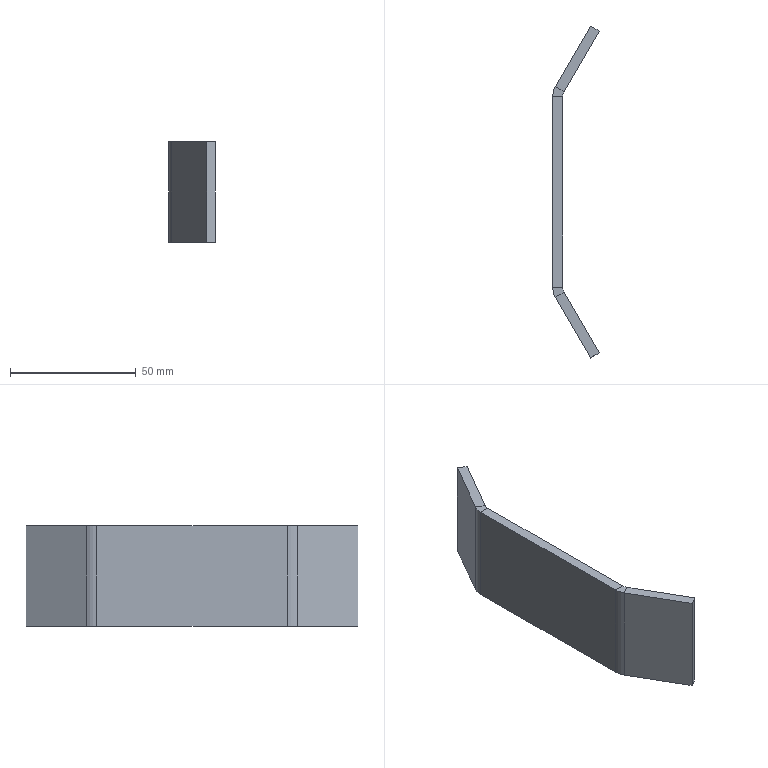Part | STEP file | 01-Bent plate 1 | 1 solid | 22 faces | box 18.464 x 131.962 x 40 mm | volume 22033 mm3 | plane 18 | cylinder 4 | commonest cylinder face diameters 8 x2 16 x2
STEP:
#1=CARTESIAN_POINT('',(0.,0.,0.));
#2=DIRECTION('',(0.,0.,1.));
#3=DIRECTION('',(1.,0.,0.));
#4=AXIS2_PLACEMENT_3D('',#1,#2,#3);
#5=CARTESIAN_POINT('',(-13.928,-24.124,40.));
#6=VERTEX_POINT('',#5);
#7=CARTESIAN_POINT('',(-10.464,-26.124,40.));
#8=VERTEX_POINT('',#7);
#9=CARTESIAN_POINT('',(-13.928,-24.124,40.));
#10=DIRECTION('',(0.866,-0.5,0.));
#11=VECTOR('',#10,1.);
#12=LINE('',#9,#11);
#13=CARTESIAN_POINT('',(-13.928,-24.124,40.));
#14=DIRECTION('',(0.,0.,1.));
#15=DIRECTION('',(1.,0.,0.));
#16=AXIS2_PLACEMENT_3D('',#13,#14,#15);
#17=PLANE('',#16);
#18=CARTESIAN_POINT('',(0.,0.));
#19=DIRECTION('',(0.866,-0.5));
#20=VECTOR('',#19,1.);
#21=LINE('',#18,#20);
#22=(GEOMETRIC_REPRESENTATION_CONTEXT(2)PARAMETRIC_REPRESENTATION_CONTEXT()REPRESENTATION_CONTEXT('',''));
#23=DEFINITIONAL_REPRESENTATION('',(#21),#22);
#24=PCURVE('',#17,#23);
#25=CARTESIAN_POINT('',(-11.,-28.124,40.));
#26=DIRECTION('',(0.,0.,1.));
#27=DIRECTION('',(1.,0.,0.));
#28=AXIS2_PLACEMENT_3D('',#25,#26,#27);
#29=PLANE('',#28);
#30=CARTESIAN_POINT('',(-2.928,4.));
#31=DIRECTION('',(0.866,-0.5));
#32=VECTOR('',#31,1.);
#33=LINE('',#30,#32);
#34=(GEOMETRIC_REPRESENTATION_CONTEXT(2)PARAMETRIC_REPRESENTATION_CONTEXT()REPRESENTATION_CONTEXT('',''));
#35=DEFINITIONAL_REPRESENTATION('',(#33),#34);
#36=PCURVE('',#29,#35);
#37=SURFACE_CURVE('',#12,(#24,#36),.PCURVE_S1.);
#38=EDGE_CURVE('',#6,#8,#37,.T.);
#39=ORIENTED_EDGE('',*,*,#38,.F.);
#40=CARTESIAN_POINT('',(-15.,-28.124,40.));
#41=VERTEX_POINT('',#40);
#42=CARTESIAN_POINT('',(-7.,-28.124,40.));
#43=DIRECTION('',(0.,0.,1.));
#44=DIRECTION('',(-1.,0.,0.));
#45=AXIS2_PLACEMENT_3D('',#42,#43,#44);
#46=CIRCLE('',#45,8.);
#47=CARTESIAN_POINT('',(6.928,-4.));
#48=DIRECTION('',(-1.,0.));
#49=AXIS2_PLACEMENT_2D('',#47,#48);
#50=CIRCLE('',#49,8.);
#51=(GEOMETRIC_REPRESENTATION_CONTEXT(2)PARAMETRIC_REPRESENTATION_CONTEXT()REPRESENTATION_CONTEXT('',''));
#52=DEFINITIONAL_REPRESENTATION('',(#50),#51);
#53=PCURVE('',#17,#52);
#54=CARTESIAN_POINT('',(-7.,-28.124,40.));
#55=DIRECTION('',(0.,0.,-1.));
#56=DIRECTION('',(-1.,0.,0.));
#57=AXIS2_PLACEMENT_3D('',#54,#55,#56);
#58=CYLINDRICAL_SURFACE('',#57,8.);
#59=CARTESIAN_POINT('',(6.283,0.));
#60=DIRECTION('',(-1.,0.));
#61=VECTOR('',#60,1.);
#62=LINE('',#59,#61);
#63=(GEOMETRIC_REPRESENTATION_CONTEXT(2)PARAMETRIC_REPRESENTATION_CONTEXT()REPRESENTATION_CONTEXT('',''));
#64=DEFINITIONAL_REPRESENTATION('',(#62),#63);
#65=PCURVE('',#58,#64);
#66=SURFACE_CURVE('',#46,(#53,#65),.PCURVE_S1.);
#67=EDGE_CURVE('',#6,#41,#66,.T.);
#68=ORIENTED_EDGE('',*,*,#67,.T.);
#69=CARTESIAN_POINT('',(-11.,-28.124,40.));
#70=VERTEX_POINT('',#69);
#71=CARTESIAN_POINT('',(-11.,-28.124,40.));
#72=DIRECTION('',(-1.,0.,0.));
#73=VECTOR('',#72,1.);
#74=LINE('',#71,#73);
#75=CARTESIAN_POINT('',(2.928,-4.));
#76=DIRECTION('',(-1.,0.));
#77=VECTOR('',#76,1.);
#78=LINE('',#75,#77);
#79=(GEOMETRIC_REPRESENTATION_CONTEXT(2)PARAMETRIC_REPRESENTATION_CONTEXT()REPRESENTATION_CONTEXT('',''));
#80=DEFINITIONAL_REPRESENTATION('',(#78),#79);
#81=PCURVE('',#17,#80);
#82=CARTESIAN_POINT('',(-10.464,-105.837,40.));
#83=DIRECTION('',(0.,0.,1.));
#84=DIRECTION('',(1.,0.,0.));
#85=AXIS2_PLACEMENT_3D('',#82,#83,#84);
#86=PLANE('',#85);
#87=CARTESIAN_POINT('',(-0.5359,77.713));
#88=DIRECTION('',(-1.,0.));
#89=VECTOR('',#88,1.);
#90=LINE('',#87,#89);
#91=(GEOMETRIC_REPRESENTATION_CONTEXT(2)PARAMETRIC_REPRESENTATION_CONTEXT()REPRESENTATION_CONTEXT('',''));
#92=DEFINITIONAL_REPRESENTATION('',(#90),#91);
#93=PCURVE('',#86,#92);
#94=SURFACE_CURVE('',#74,(#81,#93),.PCURVE_S1.);
#95=EDGE_CURVE('',#70,#41,#94,.T.);
#96=ORIENTED_EDGE('',*,*,#95,.F.);
#97=CARTESIAN_POINT('',(-7.,-28.124,40.));
#98=DIRECTION('',(0.,0.,1.));
#99=DIRECTION('',(1.,0.,0.));
#100=AXIS2_PLACEMENT_3D('',#97,#98,#99);
#101=CIRCLE('',#100,4.);
#102=CARTESIAN_POINT('',(6.928,-4.));
#103=DIRECTION('',(1.,0.));
#104=AXIS2_PLACEMENT_2D('',#102,#103);
#105=CIRCLE('',#104,4.);
#106=(GEOMETRIC_REPRESENTATION_CONTEXT(2)PARAMETRIC_REPRESENTATION_CONTEXT()REPRESENTATION_CONTEXT('',''));
#107=DEFINITIONAL_REPRESENTATION('',(#105),#106);
#108=PCURVE('',#17,#107);
#109=CARTESIAN_POINT('',(-7.,-28.124,40.));
#110=DIRECTION('',(0.,0.,-1.));
#111=DIRECTION('',(-1.,0.,0.));
#112=AXIS2_PLACEMENT_3D('',#109,#110,#111);
#113=CYLINDRICAL_SURFACE('',#112,4.);
#114=CARTESIAN_POINT('',(3.142,0.));
#115=DIRECTION('',(-1.,0.));
#116=VECTOR('',#115,1.);
#117=LINE('',#114,#116);
#118=(GEOMETRIC_REPRESENTATION_CONTEXT(2)PARAMETRIC_REPRESENTATION_CONTEXT()REPRESENTATION_CONTEXT('',''));
#119=DEFINITIONAL_REPRESENTATION('',(#117),#118);
#120=PCURVE('',#113,#119);
#121=SURFACE_CURVE('',#101,(#108,#120),.PCURVE_S1.);
#122=EDGE_CURVE('',#8,#70,#121,.T.);
#123=ORIENTED_EDGE('',*,*,#122,.F.);
#124=EDGE_LOOP('',(#39,#68,#96,#123));
#125=FACE_BOUND('',#124,.T.);
#126=ADVANCED_FACE('',(#125),#17,.T.);
#127=CARTESIAN_POINT('',(0.,0.,40.));
#128=VERTEX_POINT('',#127);
#129=CARTESIAN_POINT('',(0.,0.,40.));
#130=DIRECTION('',(-0.5,-0.866,0.));
#131=VECTOR('',#130,1.);
#132=LINE('',#129,#131);
#133=CARTESIAN_POINT('',(11.,28.124));
#134=DIRECTION('',(-0.5,-0.866));
#135=VECTOR('',#134,1.);
#136=LINE('',#133,#135);
#137=(GEOMETRIC_REPRESENTATION_CONTEXT(2)PARAMETRIC_REPRESENTATION_CONTEXT()REPRESENTATION_CONTEXT('',''));
#138=DEFINITIONAL_REPRESENTATION('',(#136),#137);
#139=PCURVE('',#29,#138);
#140=CARTESIAN_POINT('',(0.,0.,40.));
#141=DIRECTION('',(0.866,-0.5,0.));
#142=DIRECTION('',(0.5,0.866,0.));
#143=AXIS2_PLACEMENT_3D('',#140,#141,#142);
#144=PLANE('',#143);
#145=CARTESIAN_POINT('',(0.,0.));
#146=DIRECTION('',(-1.,0.));
#147=VECTOR('',#146,1.);
#148=LINE('',#145,#147);
#149=(GEOMETRIC_REPRESENTATION_CONTEXT(2)PARAMETRIC_REPRESENTATION_CONTEXT()REPRESENTATION_CONTEXT('',''));
#150=DEFINITIONAL_REPRESENTATION('',(#148),#149);
#151=PCURVE('',#144,#150);
#152=SURFACE_CURVE('',#132,(#139,#151),.PCURVE_S1.);
#153=EDGE_CURVE('',#128,#6,#152,.T.);
#154=ORIENTED_EDGE('',*,*,#153,.T.);
#155=ORIENTED_EDGE('',*,*,#38,.T.);
#156=CARTESIAN_POINT('',(3.464,-2.,40.));
#157=VERTEX_POINT('',#156);
#158=CARTESIAN_POINT('',(3.464,-2.,40.));
#159=DIRECTION('',(-0.5,-0.866,0.));
#160=VECTOR('',#159,1.);
#161=LINE('',#158,#160);
#162=CARTESIAN_POINT('',(14.464,26.124));
#163=DIRECTION('',(-0.5,-0.866));
#164=VECTOR('',#163,1.);
#165=LINE('',#162,#164);
#166=(GEOMETRIC_REPRESENTATION_CONTEXT(2)PARAMETRIC_REPRESENTATION_CONTEXT()REPRESENTATION_CONTEXT('',''));
#167=DEFINITIONAL_REPRESENTATION('',(#165),#166);
#168=PCURVE('',#29,#167);
#169=CARTESIAN_POINT('',(3.464,-2.,40.));
#170=DIRECTION('',(0.866,-0.5,0.));
#171=DIRECTION('',(0.5,0.866,0.));
#172=AXIS2_PLACEMENT_3D('',#169,#170,#171);
#173=PLANE('',#172);
#174=CARTESIAN_POINT('',(0.,0.));
#175=DIRECTION('',(-1.,0.));
#176=VECTOR('',#175,1.);
#177=LINE('',#174,#176);
#178=(GEOMETRIC_REPRESENTATION_CONTEXT(2)PARAMETRIC_REPRESENTATION_CONTEXT()REPRESENTATION_CONTEXT('',''));
#179=DEFINITIONAL_REPRESENTATION('',(#177),#178);
#180=PCURVE('',#173,#179);
#181=SURFACE_CURVE('',#161,(#168,#180),.PCURVE_S1.);
#182=EDGE_CURVE('',#157,#8,#181,.T.);
#183=ORIENTED_EDGE('',*,*,#182,.F.);
#184=CARTESIAN_POINT('',(0.,0.,40.));
#185=DIRECTION('',(0.866,-0.5,0.));
#186=VECTOR('',#185,1.);
#187=LINE('',#184,#186);
#188=CARTESIAN_POINT('',(11.,28.124));
#189=DIRECTION('',(0.866,-0.5));
#190=VECTOR('',#189,1.);
#191=LINE('',#188,#190);
#192=(GEOMETRIC_REPRESENTATION_CONTEXT(2)PARAMETRIC_REPRESENTATION_CONTEXT()REPRESENTATION_CONTEXT('',''));
#193=DEFINITIONAL_REPRESENTATION('',(#191),#192);
#194=PCURVE('',#29,#193);
#195=CARTESIAN_POINT('',(0.,0.,40.));
#196=DIRECTION('',(0.5,0.866,0.));
#197=DIRECTION('',(-0.866,0.5,0.));
#198=AXIS2_PLACEMENT_3D('',#195,#196,#197);
#199=PLANE('',#198);
#200=CARTESIAN_POINT('',(0.,0.));
#201=DIRECTION('',(-1.,0.));
#202=VECTOR('',#201,1.);
#203=LINE('',#200,#202);
#204=(GEOMETRIC_REPRESENTATION_CONTEXT(2)PARAMETRIC_REPRESENTATION_CONTEXT()REPRESENTATION_CONTEXT('',''));
#205=DEFINITIONAL_REPRESENTATION('',(#203),#204);
#206=PCURVE('',#199,#205);
#207=SURFACE_CURVE('',#187,(#194,#206),.PCURVE_S1.);
#208=EDGE_CURVE('',#128,#157,#207,.T.);
#209=ORIENTED_EDGE('',*,*,#208,.F.);
#210=EDGE_LOOP('',(#154,#155,#183,#209));
#211=FACE_BOUND('',#210,.T.);
#212=ADVANCED_FACE('',(#211),#29,.T.);
#213=CARTESIAN_POINT('',(-15.,-28.124,0.));
#214=VERTEX_POINT('',#213);
#215=CARTESIAN_POINT('',(-11.,-28.124,0.));
#216=VERTEX_POINT('',#215);
#217=CARTESIAN_POINT('',(-15.,-28.124,0.));
#218=DIRECTION('',(1.,0.,0.));
#219=VECTOR('',#218,1.);
#220=LINE('',#217,#219);
#221=CARTESIAN_POINT('',(-15.,-28.124,0.));
#222=DIRECTION('',(0.,0.,-1.));
#223=DIRECTION('',(-1.,0.,0.));
#224=AXIS2_PLACEMENT_3D('',#221,#222,#223);
#225=PLANE('',#224);
#226=CARTESIAN_POINT('',(0.,0.));
#227=DIRECTION('',(-1.,0.));
#228=VECTOR('',#227,1.);
#229=LINE('',#226,#228);
#230=(GEOMETRIC_REPRESENTATION_CONTEXT(2)PARAMETRIC_REPRESENTATION_CONTEXT()REPRESENTATION_CONTEXT('',''));
#231=DEFINITIONAL_REPRESENTATION('',(#229),#230);
#232=PCURVE('',#225,#231);
#233=CARTESIAN_POINT('',(-10.464,-26.124,0.));
#234=DIRECTION('',(0.,0.,-1.));
#235=DIRECTION('',(-1.,0.,0.));
#236=AXIS2_PLACEMENT_3D('',#233,#234,#235);
#237=PLANE('',#236);
#238=CARTESIAN_POINT('',(4.536,-2.));
#239=DIRECTION('',(-1.,0.));
#240=VECTOR('',#239,1.);
#241=LINE('',#238,#240);
#242=(GEOMETRIC_REPRESENTATION_CONTEXT(2)PARAMETRIC_REPRESENTATION_CONTEXT()REPRESENTATION_CONTEXT('',''));
#243=DEFINITIONAL_REPRESENTATION('',(#241),#242);
#244=PCURVE('',#237,#243);
#245=SURFACE_CURVE('',#220,(#232,#244),.PCURVE_S1.);
#246=EDGE_CURVE('',#214,#216,#245,.T.);
#247=ORIENTED_EDGE('',*,*,#246,.F.);
#248=CARTESIAN_POINT('',(-13.928,-24.124,0.));
#249=VERTEX_POINT('',#248);
#250=CARTESIAN_POINT('',(-7.,-28.124,0.));
#251=DIRECTION('',(0.,0.,1.));
#252=DIRECTION('',(-1.,0.,0.));
#253=AXIS2_PLACEMENT_3D('',#250,#251,#252);
#254=CIRCLE('',#253,8.);
#255=CARTESIAN_POINT('',(0.,0.));
#256=CARTESIAN_POINT('',(0.,-13.856));
#257=CARTESIAN_POINT('',(-12.,-6.928));
#258=CARTESIAN_POINT('',(-24.,0.));
#259=CARTESIAN_POINT('',(-12.,6.928));
#260=CARTESIAN_POINT('',(0.,13.856));
#261=CARTESIAN_POINT('',(0.,0.));
#262=(BOUNDED_CURVE()B_SPLINE_CURVE(2,(#255,#256,#257,#258,#259,#260,#261),.UNSPECIFIED.,.T.,.F.)B_SPLINE_CURVE_WITH_KNOTS((1,2,2,2,2,1),(-2.094,0.,2.094,4.189,6.283,8.378),.UNSPECIFIED.)CURVE()GEOMETRIC_REPRESENTATION_ITEM()RATIONAL_B_SPLINE_CURVE((1.,0.5,1.,0.5,1.,0.5,1.))REPRESENTATION_ITEM(''));
#263=(GEOMETRIC_REPRESENTATION_CONTEXT(2)PARAMETRIC_REPRESENTATION_CONTEXT()REPRESENTATION_CONTEXT('',''));
#264=DEFINITIONAL_REPRESENTATION('',(#262),#263);
#265=PCURVE('',#225,#264);
#266=CARTESIAN_POINT('',(6.283,40.));
#267=DIRECTION('',(-1.,0.));
#268=VECTOR('',#267,1.);
#269=LINE('',#266,#268);
#270=(GEOMETRIC_REPRESENTATION_CONTEXT(2)PARAMETRIC_REPRESENTATION_CONTEXT()REPRESENTATION_CONTEXT('',''));
#271=DEFINITIONAL_REPRESENTATION('',(#269),#270);
#272=PCURVE('',#58,#271);
#273=SURFACE_CURVE('',#254,(#265,#272),.PCURVE_S1.);
#274=EDGE_CURVE('',#249,#214,#273,.T.);
#275=ORIENTED_EDGE('',*,*,#274,.F.);
#276=CARTESIAN_POINT('',(-10.464,-26.124,0.));
#277=VERTEX_POINT('',#276);
#278=CARTESIAN_POINT('',(-10.464,-26.124,0.));
#279=DIRECTION('',(-0.866,0.5,0.));
#280=VECTOR('',#279,1.);
#281=LINE('',#278,#280);
#282=CARTESIAN_POINT('',(-4.536,2.));
#283=DIRECTION('',(0.866,0.5));
#284=VECTOR('',#283,1.);
#285=LINE('',#282,#284);
#286=(GEOMETRIC_REPRESENTATION_CONTEXT(2)PARAMETRIC_REPRESENTATION_CONTEXT()REPRESENTATION_CONTEXT('',''));
#287=DEFINITIONAL_REPRESENTATION('',(#285),#286);
#288=PCURVE('',#225,#287);
#289=CARTESIAN_POINT('',(-7.,-103.837,0.));
#290=DIRECTION('',(0.,0.,1.));
#291=DIRECTION('',(1.,0.,0.));
#292=AXIS2_PLACEMENT_3D('',#289,#290,#291);
#293=PLANE('',#292);
#294=CARTESIAN_POINT('',(-3.464,77.713));
#295=DIRECTION('',(-0.866,0.5));
#296=VECTOR('',#295,1.);
#297=LINE('',#294,#296);
#298=(GEOMETRIC_REPRESENTATION_CONTEXT(2)PARAMETRIC_REPRESENTATION_CONTEXT()REPRESENTATION_CONTEXT('',''));
#299=DEFINITIONAL_REPRESENTATION('',(#297),#298);
#300=PCURVE('',#293,#299);
#301=SURFACE_CURVE('',#281,(#288,#300),.PCURVE_S1.);
#302=EDGE_CURVE('',#277,#249,#301,.T.);
#303=ORIENTED_EDGE('',*,*,#302,.F.);
#304=CARTESIAN_POINT('',(-7.,-28.124,0.));
#305=DIRECTION('',(0.,0.,1.));
#306=DIRECTION('',(1.,0.,0.));
#307=AXIS2_PLACEMENT_3D('',#304,#305,#306);
#308=CIRCLE('',#307,4.);
#309=CARTESIAN_POINT('',(-12.,0.));
#310=CARTESIAN_POINT('',(-12.,6.928));
#311=CARTESIAN_POINT('',(-6.,3.464));
#312=CARTESIAN_POINT('',(0.,0.));
#313=CARTESIAN_POINT('',(-6.,-3.464));
#314=CARTESIAN_POINT('',(-12.,-6.928));
#315=CARTESIAN_POINT('',(-12.,0.));
#316=(BOUNDED_CURVE()B_SPLINE_CURVE(2,(#309,#310,#311,#312,#313,#314,#315),.UNSPECIFIED.,.T.,.F.)B_SPLINE_CURVE_WITH_KNOTS((1,2,2,2,2,1),(-2.094,0.,2.094,4.189,6.283,8.378),.UNSPECIFIED.)CURVE()GEOMETRIC_REPRESENTATION_ITEM()RATIONAL_B_SPLINE_CURVE((1.,0.5,1.,0.5,1.,0.5,1.))REPRESENTATION_ITEM(''));
#317=(GEOMETRIC_REPRESENTATION_CONTEXT(2)PARAMETRIC_REPRESENTATION_CONTEXT()REPRESENTATION_CONTEXT('',''));
#318=DEFINITIONAL_REPRESENTATION('',(#316),#317);
#319=PCURVE('',#225,#318);
#320=CARTESIAN_POINT('',(3.142,40.));
#321=DIRECTION('',(-1.,0.));
#322=VECTOR('',#321,1.);
#323=LINE('',#320,#322);
#324=(GEOMETRIC_REPRESENTATION_CONTEXT(2)PARAMETRIC_REPRESENTATION_CONTEXT()REPRESENTATION_CONTEXT('',''));
#325=DEFINITIONAL_REPRESENTATION('',(#323),#324);
#326=PCURVE('',#113,#325);
#327=SURFACE_CURVE('',#308,(#319,#326),.PCURVE_S1.);
#328=EDGE_CURVE('',#277,#216,#327,.T.);
#329=ORIENTED_EDGE('',*,*,#328,.T.);
#330=EDGE_LOOP('',(#247,#275,#303,#329));
#331=FACE_BOUND('',#330,.T.);
#332=ADVANCED_FACE('',(#331),#225,.T.);
#333=CARTESIAN_POINT('',(-15.,-103.837,0.));
#334=VERTEX_POINT('',#333);
#335=CARTESIAN_POINT('',(-15.,-25.981,0.));
#336=DIRECTION('',(0.,-1.,0.));
#337=VECTOR('',#336,1.);
#338=LINE('',#335,#337);
#339=CARTESIAN_POINT('',(4.536,0.1436));
#340=DIRECTION('',(0.,-1.));
#341=VECTOR('',#340,1.);
#342=LINE('',#339,#341);
#343=(GEOMETRIC_REPRESENTATION_CONTEXT(2)PARAMETRIC_REPRESENTATION_CONTEXT()REPRESENTATION_CONTEXT('',''));
#344=DEFINITIONAL_REPRESENTATION('',(#342),#343);
#345=PCURVE('',#237,#344);
#346=CARTESIAN_POINT('',(-15.,-25.981,40.));
#347=DIRECTION('',(1.,0.,0.));
#348=DIRECTION('',(0.,1.,0.));
#349=AXIS2_PLACEMENT_3D('',#346,#347,#348);
#350=PLANE('',#349);
#351=CARTESIAN_POINT('',(0.,-40.));
#352=DIRECTION('',(-1.,0.));
#353=VECTOR('',#352,1.);
#354=LINE('',#351,#353);
#355=(GEOMETRIC_REPRESENTATION_CONTEXT(2)PARAMETRIC_REPRESENTATION_CONTEXT()REPRESENTATION_CONTEXT('',''));
#356=DEFINITIONAL_REPRESENTATION('',(#354),#355);
#357=PCURVE('',#350,#356);
#358=SURFACE_CURVE('',#338,(#345,#357),.PCURVE_S1.);
#359=EDGE_CURVE('',#214,#334,#358,.T.);
#360=ORIENTED_EDGE('',*,*,#359,.F.);
#361=ORIENTED_EDGE('',*,*,#246,.T.);
#362=CARTESIAN_POINT('',(-11.,-103.837,0.));
#363=VERTEX_POINT('',#362);
#364=CARTESIAN_POINT('',(-11.,-25.981,0.));
#365=DIRECTION('',(0.,-1.,0.));
#366=VECTOR('',#365,1.);
#367=LINE('',#364,#366);
#368=CARTESIAN_POINT('',(0.5359,0.1436));
#369=DIRECTION('',(0.,-1.));
#370=VECTOR('',#369,1.);
#371=LINE('',#368,#370);
#372=(GEOMETRIC_REPRESENTATION_CONTEXT(2)PARAMETRIC_REPRESENTATION_CONTEXT()REPRESENTATION_CONTEXT('',''));
#373=DEFINITIONAL_REPRESENTATION('',(#371),#372);
#374=PCURVE('',#237,#373);
#375=CARTESIAN_POINT('',(-11.,-25.981,40.));
#376=DIRECTION('',(1.,0.,0.));
#377=DIRECTION('',(0.,1.,0.));
#378=AXIS2_PLACEMENT_3D('',#375,#376,#377);
#379=PLANE('',#378);
#380=CARTESIAN_POINT('',(0.,-40.));
#381=DIRECTION('',(-1.,0.));
#382=VECTOR('',#381,1.);
#383=LINE('',#380,#382);
#384=(GEOMETRIC_REPRESENTATION_CONTEXT(2)PARAMETRIC_REPRESENTATION_CONTEXT()REPRESENTATION_CONTEXT('',''));
#385=DEFINITIONAL_REPRESENTATION('',(#383),#384);
#386=PCURVE('',#379,#385);
#387=SURFACE_CURVE('',#367,(#374,#386),.PCURVE_S1.);
#388=EDGE_CURVE('',#216,#363,#387,.T.);
#389=ORIENTED_EDGE('',*,*,#388,.T.);
#390=CARTESIAN_POINT('',(-11.,-103.837,0.));
#391=DIRECTION('',(-1.,0.,0.));
#392=VECTOR('',#391,1.);
#393=LINE('',#390,#392);
#394=CARTESIAN_POINT('',(0.5359,-77.713));
#395=DIRECTION('',(1.,0.));
#396=VECTOR('',#395,1.);
#397=LINE('',#394,#396);
#398=(GEOMETRIC_REPRESENTATION_CONTEXT(2)PARAMETRIC_REPRESENTATION_CONTEXT()REPRESENTATION_CONTEXT('',''));
#399=DEFINITIONAL_REPRESENTATION('',(#397),#398);
#400=PCURVE('',#237,#399);
#401=CARTESIAN_POINT('',(-13.928,-107.837,0.));
#402=DIRECTION('',(0.,0.,-1.));
#403=DIRECTION('',(-1.,0.,0.));
#404=AXIS2_PLACEMENT_3D('',#401,#402,#403);
#405=PLANE('',#404);
#406=CARTESIAN_POINT('',(-2.928,4.));
#407=DIRECTION('',(1.,0.));
#408=VECTOR('',#407,1.);
#409=LINE('',#406,#408);
#410=(GEOMETRIC_REPRESENTATION_CONTEXT(2)PARAMETRIC_REPRESENTATION_CONTEXT()REPRESENTATION_CONTEXT('',''));
#411=DEFINITIONAL_REPRESENTATION('',(#409),#410);
#412=PCURVE('',#405,#411);
#413=SURFACE_CURVE('',#393,(#400,#412),.PCURVE_S1.);
#414=EDGE_CURVE('',#363,#334,#413,.T.);
#415=ORIENTED_EDGE('',*,*,#414,.T.);
#416=EDGE_LOOP('',(#360,#361,#389,#415));
#417=FACE_BOUND('',#416,.T.);
#418=ADVANCED_FACE('',(#417),#237,.T.);
#419=CARTESIAN_POINT('',(-15.,-103.837,40.));
#420=VERTEX_POINT('',#419);
#421=CARTESIAN_POINT('',(-11.,-103.837,40.));
#422=VERTEX_POINT('',#421);
#423=CARTESIAN_POINT('',(-15.,-103.837,40.));
#424=DIRECTION('',(1.,0.,0.));
#425=VECTOR('',#424,1.);
#426=LINE('',#423,#425);
#427=CARTESIAN_POINT('',(-15.,-103.837,40.));
#428=DIRECTION('',(0.,0.,1.));
#429=DIRECTION('',(1.,0.,0.));
#430=AXIS2_PLACEMENT_3D('',#427,#428,#429);
#431=PLANE('',#430);
#432=CARTESIAN_POINT('',(0.,0.));
#433=DIRECTION('',(1.,0.));
#434=VECTOR('',#433,1.);
#435=LINE('',#432,#434);
#436=(GEOMETRIC_REPRESENTATION_CONTEXT(2)PARAMETRIC_REPRESENTATION_CONTEXT()REPRESENTATION_CONTEXT('',''));
#437=DEFINITIONAL_REPRESENTATION('',(#435),#436);
#438=PCURVE('',#431,#437);
#439=CARTESIAN_POINT('',(-4.536,2.));
#440=DIRECTION('',(1.,0.));
#441=VECTOR('',#440,1.);
#442=LINE('',#439,#441);
#443=(GEOMETRIC_REPRESENTATION_CONTEXT(2)PARAMETRIC_REPRESENTATION_CONTEXT()REPRESENTATION_CONTEXT('',''));
#444=DEFINITIONAL_REPRESENTATION('',(#442),#443);
#445=PCURVE('',#86,#444);
#446=SURFACE_CURVE('',#426,(#438,#445),.PCURVE_S1.);
#447=EDGE_CURVE('',#420,#422,#446,.T.);
#448=ORIENTED_EDGE('',*,*,#447,.F.);
#449=CARTESIAN_POINT('',(-13.928,-107.837,40.));
#450=VERTEX_POINT('',#449);
#451=CARTESIAN_POINT('',(-7.,-103.837,40.));
#452=DIRECTION('',(0.,0.,1.));
#453=DIRECTION('',(-1.,0.,0.));
#454=AXIS2_PLACEMENT_3D('',#451,#452,#453);
#455=CIRCLE('',#454,8.);
#456=CARTESIAN_POINT('',(8.,0.));
#457=DIRECTION('',(-1.,0.));
#458=AXIS2_PLACEMENT_2D('',#456,#457);
#459=CIRCLE('',#458,8.);
#460=(GEOMETRIC_REPRESENTATION_CONTEXT(2)PARAMETRIC_REPRESENTATION_CONTEXT()REPRESENTATION_CONTEXT('',''));
#461=DEFINITIONAL_REPRESENTATION('',(#459),#460);
#462=PCURVE('',#431,#461);
#463=CARTESIAN_POINT('',(-7.,-103.837,40.));
#464=DIRECTION('',(0.,0.,-1.));
#465=DIRECTION('',(-1.,0.,0.));
#466=AXIS2_PLACEMENT_3D('',#463,#464,#465);
#467=CYLINDRICAL_SURFACE('',#466,8.);
#468=CARTESIAN_POINT('',(6.283,0.));
#469=DIRECTION('',(-1.,0.));
#470=VECTOR('',#469,1.);
#471=LINE('',#468,#470);
#472=(GEOMETRIC_REPRESENTATION_CONTEXT(2)PARAMETRIC_REPRESENTATION_CONTEXT()REPRESENTATION_CONTEXT('',''));
#473=DEFINITIONAL_REPRESENTATION('',(#471),#472);
#474=PCURVE('',#467,#473);
#475=SURFACE_CURVE('',#455,(#462,#474),.PCURVE_S1.);
#476=EDGE_CURVE('',#420,#450,#475,.T.);
#477=ORIENTED_EDGE('',*,*,#476,.T.);
#478=CARTESIAN_POINT('',(-10.464,-105.837,40.));
#479=VERTEX_POINT('',#478);
#480=CARTESIAN_POINT('',(-10.464,-105.837,40.));
#481=DIRECTION('',(-0.866,-0.5,0.));
#482=VECTOR('',#481,1.);
#483=LINE('',#480,#482);
#484=CARTESIAN_POINT('',(4.536,-2.));
#485=DIRECTION('',(-0.866,-0.5));
#486=VECTOR('',#485,1.);
#487=LINE('',#484,#486);
#488=(GEOMETRIC_REPRESENTATION_CONTEXT(2)PARAMETRIC_REPRESENTATION_CONTEXT()REPRESENTATION_CONTEXT('',''));
#489=DEFINITIONAL_REPRESENTATION('',(#487),#488);
#490=PCURVE('',#431,#489);
#491=CARTESIAN_POINT('',(-7.,-103.837,40.));
#492=DIRECTION('',(0.,0.,1.));
#493=DIRECTION('',(1.,0.,0.));
#494=AXIS2_PLACEMENT_3D('',#491,#492,#493);
#495=PLANE('',#494);
#496=CARTESIAN_POINT('',(-3.464,-2.));
#497=DIRECTION('',(-0.866,-0.5));
#498=VECTOR('',#497,1.);
#499=LINE('',#496,#498);
#500=(GEOMETRIC_REPRESENTATION_CONTEXT(2)PARAMETRIC_REPRESENTATION_CONTEXT()REPRESENTATION_CONTEXT('',''));
#501=DEFINITIONAL_REPRESENTATION('',(#499),#500);
#502=PCURVE('',#495,#501);
#503=SURFACE_CURVE('',#483,(#490,#502),.PCURVE_S1.);
#504=EDGE_CURVE('',#479,#450,#503,.T.);
#505=ORIENTED_EDGE('',*,*,#504,.F.);
#506=CARTESIAN_POINT('',(-7.,-103.837,40.));
#507=DIRECTION('',(0.,0.,1.));
#508=DIRECTION('',(1.,0.,0.));
#509=AXIS2_PLACEMENT_3D('',#506,#507,#508);
#510=CIRCLE('',#509,4.);
#511=CARTESIAN_POINT('',(8.,0.));
#512=DIRECTION('',(1.,0.));
#513=AXIS2_PLACEMENT_2D('',#511,#512);
#514=CIRCLE('',#513,4.);
#515=(GEOMETRIC_REPRESENTATION_CONTEXT(2)PARAMETRIC_REPRESENTATION_CONTEXT()REPRESENTATION_CONTEXT('',''));
#516=DEFINITIONAL_REPRESENTATION('',(#514),#515);
#517=PCURVE('',#431,#516);
#518=CARTESIAN_POINT('',(-7.,-103.837,40.));
#519=DIRECTION('',(0.,0.,-1.));
#520=DIRECTION('',(-1.,0.,0.));
#521=AXIS2_PLACEMENT_3D('',#518,#519,#520);
#522=CYLINDRICAL_SURFACE('',#521,4.);
#523=CARTESIAN_POINT('',(9.425,0.));
#524=DIRECTION('',(-1.,0.));
#525=VECTOR('',#524,1.);
#526=LINE('',#523,#525);
#527=(GEOMETRIC_REPRESENTATION_CONTEXT(2)PARAMETRIC_REPRESENTATION_CONTEXT()REPRESENTATION_CONTEXT('',''));
#528=DEFINITIONAL_REPRESENTATION('',(#526),#527);
#529=PCURVE('',#522,#528);
#530=SURFACE_CURVE('',#510,(#517,#529),.PCURVE_S1.);
#531=EDGE_CURVE('',#422,#479,#530,.T.);
#532=ORIENTED_EDGE('',*,*,#531,.F.);
#533=EDGE_LOOP('',(#448,#477,#505,#532));
#534=FACE_BOUND('',#533,.T.);
#535=ADVANCED_FACE('',(#534),#431,.T.);
#536=CARTESIAN_POINT('',(-15.,-25.981,40.));
#537=DIRECTION('',(0.,-1.,0.));
#538=VECTOR('',#537,1.);
#539=LINE('',#536,#538);
#540=CARTESIAN_POINT('',(-4.536,79.856));
#541=DIRECTION('',(0.,-1.));
#542=VECTOR('',#541,1.);
#543=LINE('',#540,#542);
#544=(GEOMETRIC_REPRESENTATION_CONTEXT(2)PARAMETRIC_REPRESENTATION_CONTEXT()REPRESENTATION_CONTEXT('',''));
#545=DEFINITIONAL_REPRESENTATION('',(#543),#544);
#546=PCURVE('',#86,#545);
#547=CARTESIAN_POINT('',(0.,0.));
#548=DIRECTION('',(-1.,0.));
#549=VECTOR('',#548,1.);
#550=LINE('',#547,#549);
#551=(GEOMETRIC_REPRESENTATION_CONTEXT(2)PARAMETRIC_REPRESENTATION_CONTEXT()REPRESENTATION_CONTEXT('',''));
#552=DEFINITIONAL_REPRESENTATION('',(#550),#551);
#553=PCURVE('',#350,#552);
#554=SURFACE_CURVE('',#539,(#546,#553),.PCURVE_S1.);
#555=EDGE_CURVE('',#41,#420,#554,.T.);
#556=ORIENTED_EDGE('',*,*,#555,.T.);
#557=ORIENTED_EDGE('',*,*,#447,.T.);
#558=CARTESIAN_POINT('',(-11.,-25.981,40.));
#559=DIRECTION('',(0.,-1.,0.));
#560=VECTOR('',#559,1.);
#561=LINE('',#558,#560);
#562=CARTESIAN_POINT('',(-0.5359,79.856));
#563=DIRECTION('',(0.,-1.));
#564=VECTOR('',#563,1.);
#565=LINE('',#562,#564);
#566=(GEOMETRIC_REPRESENTATION_CONTEXT(2)PARAMETRIC_REPRESENTATION_CONTEXT()REPRESENTATION_CONTEXT('',''));
#567=DEFINITIONAL_REPRESENTATION('',(#565),#566);
#568=PCURVE('',#86,#567);
#569=CARTESIAN_POINT('',(0.,0.));
#570=DIRECTION('',(-1.,0.));
#571=VECTOR('',#570,1.);
#572=LINE('',#569,#571);
#573=(GEOMETRIC_REPRESENTATION_CONTEXT(2)PARAMETRIC_REPRESENTATION_CONTEXT()REPRESENTATION_CONTEXT('',''));
#574=DEFINITIONAL_REPRESENTATION('',(#572),#573);
#575=PCURVE('',#379,#574);
#576=SURFACE_CURVE('',#561,(#568,#575),.PCURVE_S1.);
#577=EDGE_CURVE('',#70,#422,#576,.T.);
#578=ORIENTED_EDGE('',*,*,#577,.F.);
#579=ORIENTED_EDGE('',*,*,#95,.T.);
#580=EDGE_LOOP('',(#556,#557,#578,#579));
#581=FACE_BOUND('',#580,.T.);
#582=ADVANCED_FACE('',(#581),#86,.T.);
#583=CARTESIAN_POINT('',(-13.928,-107.837,0.));
#584=VERTEX_POINT('',#583);
#585=CARTESIAN_POINT('',(-10.464,-105.837,0.));
#586=VERTEX_POINT('',#585);
#587=CARTESIAN_POINT('',(-13.928,-107.837,0.));
#588=DIRECTION('',(0.866,0.5,0.));
#589=VECTOR('',#588,1.);
#590=LINE('',#587,#589);
#591=CARTESIAN_POINT('',(0.,0.));
#592=DIRECTION('',(-0.866,0.5));
#593=VECTOR('',#592,1.);
#594=LINE('',#591,#593);
#595=(GEOMETRIC_REPRESENTATION_CONTEXT(2)PARAMETRIC_REPRESENTATION_CONTEXT()REPRESENTATION_CONTEXT('',''));
#596=DEFINITIONAL_REPRESENTATION('',(#594),#595);
#597=PCURVE('',#405,#596);
#598=CARTESIAN_POINT('',(-11.,-103.837,0.));
#599=DIRECTION('',(0.,0.,-1.));
#600=DIRECTION('',(-1.,0.,0.));
#601=AXIS2_PLACEMENT_3D('',#598,#599,#600);
#602=PLANE('',#601);
#603=CARTESIAN_POINT('',(2.928,-4.));
#604=DIRECTION('',(-0.866,0.5));
#605=VECTOR('',#604,1.);
#606=LINE('',#603,#605);
#607=(GEOMETRIC_REPRESENTATION_CONTEXT(2)PARAMETRIC_REPRESENTATION_CONTEXT()REPRESENTATION_CONTEXT('',''));
#608=DEFINITIONAL_REPRESENTATION('',(#606),#607);
#609=PCURVE('',#602,#608);
#610=SURFACE_CURVE('',#590,(#597,#609),.PCURVE_S1.);
#611=EDGE_CURVE('',#584,#586,#610,.T.);
#612=ORIENTED_EDGE('',*,*,#611,.F.);
#613=CARTESIAN_POINT('',(-7.,-103.837,0.));
#614=DIRECTION('',(0.,0.,1.));
#615=DIRECTION('',(-1.,0.,0.));
#616=AXIS2_PLACEMENT_3D('',#613,#614,#615);
#617=CIRCLE('',#616,8.);
#618=CARTESIAN_POINT('',(1.072,4.));
#619=CARTESIAN_POINT('',(1.072,-9.856));
#620=CARTESIAN_POINT('',(-10.928,-2.928));
#621=CARTESIAN_POINT('',(-22.928,4.));
#622=CARTESIAN_POINT('',(-10.928,10.928));
#623=CARTESIAN_POINT('',(1.072,17.856));
#624=CARTESIAN_POINT('',(1.072,4.));
#625=(BOUNDED_CURVE()B_SPLINE_CURVE(2,(#618,#619,#620,#621,#622,#623,#624),.UNSPECIFIED.,.T.,.F.)B_SPLINE_CURVE_WITH_KNOTS((1,2,2,2,2,1),(-2.094,0.,2.094,4.189,6.283,8.378),.UNSPECIFIED.)CURVE()GEOMETRIC_REPRESENTATION_ITEM()RATIONAL_B_SPLINE_CURVE((1.,0.5,1.,0.5,1.,0.5,1.))REPRESENTATION_ITEM(''));
#626=(GEOMETRIC_REPRESENTATION_CONTEXT(2)PARAMETRIC_REPRESENTATION_CONTEXT()REPRESENTATION_CONTEXT('',''));
#627=DEFINITIONAL_REPRESENTATION('',(#625),#626);
#628=PCURVE('',#405,#627);
#629=CARTESIAN_POINT('',(6.283,40.));
#630=DIRECTION('',(-1.,0.));
#631=VECTOR('',#630,1.);
#632=LINE('',#629,#631);
#633=(GEOMETRIC_REPRESENTATION_CONTEXT(2)PARAMETRIC_REPRESENTATION_CONTEXT()REPRESENTATION_CONTEXT('',''));
#634=DEFINITIONAL_REPRESENTATION('',(#632),#633);
#635=PCURVE('',#467,#634);
#636=SURFACE_CURVE('',#617,(#628,#635),.PCURVE_S1.);
#637=EDGE_CURVE('',#334,#584,#636,.T.);
#638=ORIENTED_EDGE('',*,*,#637,.F.);
#639=ORIENTED_EDGE('',*,*,#414,.F.);
#640=CARTESIAN_POINT('',(-7.,-103.837,0.));
#641=DIRECTION('',(0.,0.,1.));
#642=DIRECTION('',(1.,0.,0.));
#643=AXIS2_PLACEMENT_3D('',#640,#641,#642);
#644=CIRCLE('',#643,4.);
#645=CARTESIAN_POINT('',(-10.928,4.));
#646=CARTESIAN_POINT('',(-10.928,10.928));
#647=CARTESIAN_POINT('',(-4.928,7.464));
#648=CARTESIAN_POINT('',(1.072,4.));
#649=CARTESIAN_POINT('',(-4.928,0.5359));
#650=CARTESIAN_POINT('',(-10.928,-2.928));
#651=CARTESIAN_POINT('',(-10.928,4.));
#652=(BOUNDED_CURVE()B_SPLINE_CURVE(2,(#645,#646,#647,#648,#649,#650,#651),.UNSPECIFIED.,.T.,.F.)B_SPLINE_CURVE_WITH_KNOTS((1,2,2,2,2,1),(-2.094,0.,2.094,4.189,6.283,8.378),.UNSPECIFIED.)CURVE()GEOMETRIC_REPRESENTATION_ITEM()RATIONAL_B_SPLINE_CURVE((1.,0.5,1.,0.5,1.,0.5,1.))REPRESENTATION_ITEM(''));
#653=(GEOMETRIC_REPRESENTATION_CONTEXT(2)PARAMETRIC_REPRESENTATION_CONTEXT()REPRESENTATION_CONTEXT('',''));
#654=DEFINITIONAL_REPRESENTATION('',(#652),#653);
#655=PCURVE('',#405,#654);
#656=CARTESIAN_POINT('',(9.425,40.));
#657=DIRECTION('',(-1.,0.));
#658=VECTOR('',#657,1.);
#659=LINE('',#656,#658);
#660=(GEOMETRIC_REPRESENTATION_CONTEXT(2)PARAMETRIC_REPRESENTATION_CONTEXT()REPRESENTATION_CONTEXT('',''));
#661=DEFINITIONAL_REPRESENTATION('',(#659),#660);
#662=PCURVE('',#522,#661);
#663=SURFACE_CURVE('',#644,(#655,#662),.PCURVE_S1.);
#664=EDGE_CURVE('',#363,#586,#663,.T.);
#665=ORIENTED_EDGE('',*,*,#664,.T.);
#666=EDGE_LOOP('',(#612,#638,#639,#665));
#667=FACE_BOUND('',#666,.T.);
#668=ADVANCED_FACE('',(#667),#405,.T.);
#669=CARTESIAN_POINT('',(0.,-131.962,0.));
#670=VERTEX_POINT('',#669);
#671=CARTESIAN_POINT('',(-15.,-105.981,0.));
#672=DIRECTION('',(0.5,-0.866,0.));
#673=VECTOR('',#672,1.);
#674=LINE('',#671,#673);
#675=CARTESIAN_POINT('',(4.,-2.144));
#676=DIRECTION('',(-0.5,-0.866));
#677=VECTOR('',#676,1.);
#678=LINE('',#675,#677);
#679=(GEOMETRIC_REPRESENTATION_CONTEXT(2)PARAMETRIC_REPRESENTATION_CONTEXT()REPRESENTATION_CONTEXT('',''));
#680=DEFINITIONAL_REPRESENTATION('',(#678),#679);
#681=PCURVE('',#602,#680);
#682=CARTESIAN_POINT('',(-15.,-105.981,40.));
#683=DIRECTION('',(0.866,0.5,0.));
#684=DIRECTION('',(-0.5,0.866,0.));
#685=AXIS2_PLACEMENT_3D('',#682,#683,#684);
#686=PLANE('',#685);
#687=CARTESIAN_POINT('',(0.,-40.));
#688=DIRECTION('',(-1.,0.));
#689=VECTOR('',#688,1.);
#690=LINE('',#687,#689);
#691=(GEOMETRIC_REPRESENTATION_CONTEXT(2)PARAMETRIC_REPRESENTATION_CONTEXT()REPRESENTATION_CONTEXT('',''));
#692=DEFINITIONAL_REPRESENTATION('',(#690),#691);
#693=PCURVE('',#686,#692);
#694=SURFACE_CURVE('',#674,(#681,#693),.PCURVE_S1.);
#695=EDGE_CURVE('',#584,#670,#694,.T.);
#696=ORIENTED_EDGE('',*,*,#695,.F.);
#697=ORIENTED_EDGE('',*,*,#611,.T.);
#698=CARTESIAN_POINT('',(3.464,-129.962,0.));
#699=VERTEX_POINT('',#698);
#700=CARTESIAN_POINT('',(-11.536,-103.981,0.));
#701=DIRECTION('',(0.5,-0.866,0.));
#702=VECTOR('',#701,1.);
#703=LINE('',#700,#702);
#704=CARTESIAN_POINT('',(0.5359,-0.1436));
#705=DIRECTION('',(-0.5,-0.866));
#706=VECTOR('',#705,1.);
#707=LINE('',#704,#706);
#708=(GEOMETRIC_REPRESENTATION_CONTEXT(2)PARAMETRIC_REPRESENTATION_CONTEXT()REPRESENTATION_CONTEXT('',''));
#709=DEFINITIONAL_REPRESENTATION('',(#707),#708);
#710=PCURVE('',#602,#709);
#711=CARTESIAN_POINT('',(-11.536,-103.981,40.));
#712=DIRECTION('',(0.866,0.5,0.));
#713=DIRECTION('',(-0.5,0.866,0.));
#714=AXIS2_PLACEMENT_3D('',#711,#712,#713);
#715=PLANE('',#714);
#716=CARTESIAN_POINT('',(0.,-40.));
#717=DIRECTION('',(-1.,0.));
#718=VECTOR('',#717,1.);
#719=LINE('',#716,#718);
#720=(GEOMETRIC_REPRESENTATION_CONTEXT(2)PARAMETRIC_REPRESENTATION_CONTEXT()REPRESENTATION_CONTEXT('',''));
#721=DEFINITIONAL_REPRESENTATION('',(#719),#720);
#722=PCURVE('',#715,#721);
#723=SURFACE_CURVE('',#703,(#710,#722),.PCURVE_S1.);
#724=EDGE_CURVE('',#586,#699,#723,.T.);
#725=ORIENTED_EDGE('',*,*,#724,.T.);
#726=CARTESIAN_POINT('',(3.464,-129.962,0.));
#727=DIRECTION('',(-0.866,-0.5,0.));
#728=VECTOR('',#727,1.);
#729=LINE('',#726,#728);
#730=CARTESIAN_POINT('',(-14.464,-26.124));
#731=DIRECTION('',(0.866,-0.5));
#732=VECTOR('',#731,1.);
#733=LINE('',#730,#732);
#734=(GEOMETRIC_REPRESENTATION_CONTEXT(2)PARAMETRIC_REPRESENTATION_CONTEXT()REPRESENTATION_CONTEXT('',''));
#735=DEFINITIONAL_REPRESENTATION('',(#733),#734);
#736=PCURVE('',#602,#735);
#737=CARTESIAN_POINT('',(3.464,-129.962,40.));
#738=DIRECTION('',(0.5,-0.866,0.));
#739=DIRECTION('',(0.866,0.5,0.));
#740=AXIS2_PLACEMENT_3D('',#737,#738,#739);
#741=PLANE('',#740);
#742=CARTESIAN_POINT('',(0.,-40.));
#743=DIRECTION('',(-1.,0.));
#744=VECTOR('',#743,1.);
#745=LINE('',#742,#744);
#746=(GEOMETRIC_REPRESENTATION_CONTEXT(2)PARAMETRIC_REPRESENTATION_CONTEXT()REPRESENTATION_CONTEXT('',''));
#747=DEFINITIONAL_REPRESENTATION('',(#745),#746);
#748=PCURVE('',#741,#747);
#749=SURFACE_CURVE('',#729,(#736,#748),.PCURVE_S1.);
#750=EDGE_CURVE('',#699,#670,#749,.T.);
#751=ORIENTED_EDGE('',*,*,#750,.T.);
#752=EDGE_LOOP('',(#696,#697,#725,#751));
#753=FACE_BOUND('',#752,.T.);
#754=ADVANCED_FACE('',(#753),#602,.T.);
#755=ORIENTED_EDGE('',*,*,#695,.T.);
#756=CARTESIAN_POINT('',(0.,-131.962,40.));
#757=VERTEX_POINT('',#756);
#758=CARTESIAN_POINT('',(0.,-131.962,40.));
#759=DIRECTION('',(0.,0.,-1.));
#760=VECTOR('',#759,1.);
#761=LINE('',#758,#760);
#762=CARTESIAN_POINT('',(-30.,0.));
#763=DIRECTION('',(0.,-1.));
#764=VECTOR('',#763,1.);
#765=LINE('',#762,#764);
#766=(GEOMETRIC_REPRESENTATION_CONTEXT(2)PARAMETRIC_REPRESENTATION_CONTEXT()REPRESENTATION_CONTEXT('',''));
#767=DEFINITIONAL_REPRESENTATION('',(#765),#766);
#768=PCURVE('',#686,#767);
#769=CARTESIAN_POINT('',(-4.,0.));
#770=DIRECTION('',(0.,-1.));
#771=VECTOR('',#770,1.);
#772=LINE('',#769,#771);
#773=(GEOMETRIC_REPRESENTATION_CONTEXT(2)PARAMETRIC_REPRESENTATION_CONTEXT()REPRESENTATION_CONTEXT('',''));
#774=DEFINITIONAL_REPRESENTATION('',(#772),#773);
#775=PCURVE('',#741,#774);
#776=SURFACE_CURVE('',#761,(#768,#775),.PCURVE_S1.);
#777=EDGE_CURVE('',#757,#670,#776,.T.);
#778=ORIENTED_EDGE('',*,*,#777,.F.);
#779=CARTESIAN_POINT('',(-15.,-105.981,40.));
#780=DIRECTION('',(0.5,-0.866,0.));
#781=VECTOR('',#780,1.);
#782=LINE('',#779,#781);
#783=CARTESIAN_POINT('',(0.,0.));
#784=DIRECTION('',(-1.,0.));
#785=VECTOR('',#784,1.);
#786=LINE('',#783,#785);
#787=(GEOMETRIC_REPRESENTATION_CONTEXT(2)PARAMETRIC_REPRESENTATION_CONTEXT()REPRESENTATION_CONTEXT('',''));
#788=DEFINITIONAL_REPRESENTATION('',(#786),#787);
#789=PCURVE('',#686,#788);
#790=CARTESIAN_POINT('',(-8.,-2.144));
#791=DIRECTION('',(0.5,-0.866));
#792=VECTOR('',#791,1.);
#793=LINE('',#790,#792);
#794=(GEOMETRIC_REPRESENTATION_CONTEXT(2)PARAMETRIC_REPRESENTATION_CONTEXT()REPRESENTATION_CONTEXT('',''));
#795=DEFINITIONAL_REPRESENTATION('',(#793),#794);
#796=PCURVE('',#495,#795);
#797=SURFACE_CURVE('',#782,(#789,#796),.PCURVE_S1.);
#798=EDGE_CURVE('',#450,#757,#797,.T.);
#799=ORIENTED_EDGE('',*,*,#798,.F.);
#800=CARTESIAN_POINT('',(-13.928,-107.837,40.));
#801=DIRECTION('',(0.,0.,-1.));
#802=VECTOR('',#801,1.);
#803=LINE('',#800,#802);
#804=CARTESIAN_POINT('',(-2.144,0.));
#805=DIRECTION('',(0.,-1.));
#806=VECTOR('',#805,1.);
#807=LINE('',#804,#806);
#808=(GEOMETRIC_REPRESENTATION_CONTEXT(2)PARAMETRIC_REPRESENTATION_CONTEXT()REPRESENTATION_CONTEXT('',''));
#809=DEFINITIONAL_REPRESENTATION('',(#807),#808);
#810=PCURVE('',#686,#809);
#811=CARTESIAN_POINT('',(5.76,0.));
#812=DIRECTION('',(0.,1.));
#813=VECTOR('',#812,1.);
#814=LINE('',#811,#813);
#815=(GEOMETRIC_REPRESENTATION_CONTEXT(2)PARAMETRIC_REPRESENTATION_CONTEXT()REPRESENTATION_CONTEXT('',''));
#816=DEFINITIONAL_REPRESENTATION('',(#814),#815);
#817=PCURVE('',#467,#816);
#818=SURFACE_CURVE('',#803,(#810,#817),.PCURVE_S1.);
#819=EDGE_CURVE('',#450,#584,#818,.T.);
#820=ORIENTED_EDGE('',*,*,#819,.T.);
#821=EDGE_LOOP('',(#755,#778,#799,#820));
#822=FACE_BOUND('',#821,.T.);
#823=ADVANCED_FACE('',(#822),#686,.F.);
#824=ORIENTED_EDGE('',*,*,#750,.F.);
#825=CARTESIAN_POINT('',(3.464,-129.962,40.));
#826=VERTEX_POINT('',#825);
#827=CARTESIAN_POINT('',(3.464,-129.962,40.));
#828=DIRECTION('',(0.,0.,-1.));
#829=VECTOR('',#828,1.);
#830=LINE('',#827,#829);
#831=CARTESIAN_POINT('',(0.,0.));
#832=DIRECTION('',(0.,-1.));
#833=VECTOR('',#832,1.);
#834=LINE('',#831,#833);
#835=(GEOMETRIC_REPRESENTATION_CONTEXT(2)PARAMETRIC_REPRESENTATION_CONTEXT()REPRESENTATION_CONTEXT('',''));
#836=DEFINITIONAL_REPRESENTATION('',(#834),#835);
#837=PCURVE('',#741,#836);
#838=CARTESIAN_POINT('',(-30.,0.));
#839=DIRECTION('',(0.,-1.));
#840=VECTOR('',#839,1.);
#841=LINE('',#838,#840);
#842=(GEOMETRIC_REPRESENTATION_CONTEXT(2)PARAMETRIC_REPRESENTATION_CONTEXT()REPRESENTATION_CONTEXT('',''));
#843=DEFINITIONAL_REPRESENTATION('',(#841),#842);
#844=PCURVE('',#715,#843);
#845=SURFACE_CURVE('',#830,(#837,#844),.PCURVE_S1.);
#846=EDGE_CURVE('',#826,#699,#845,.T.);
#847=ORIENTED_EDGE('',*,*,#846,.F.);
#848=CARTESIAN_POINT('',(3.464,-129.962,40.));
#849=DIRECTION('',(-0.866,-0.5,0.));
#850=VECTOR('',#849,1.);
#851=LINE('',#848,#850);
#852=CARTESIAN_POINT('',(0.,0.));
#853=DIRECTION('',(-1.,0.));
#854=VECTOR('',#853,1.);
#855=LINE('',#852,#854);
#856=(GEOMETRIC_REPRESENTATION_CONTEXT(2)PARAMETRIC_REPRESENTATION_CONTEXT()REPRESENTATION_CONTEXT('',''));
#857=DEFINITIONAL_REPRESENTATION('',(#855),#856);
#858=PCURVE('',#741,#857);
#859=CARTESIAN_POINT('',(10.464,-26.124));
#860=DIRECTION('',(-0.866,-0.5));
#861=VECTOR('',#860,1.);
#862=LINE('',#859,#861);
#863=(GEOMETRIC_REPRESENTATION_CONTEXT(2)PARAMETRIC_REPRESENTATION_CONTEXT()REPRESENTATION_CONTEXT('',''));
#864=DEFINITIONAL_REPRESENTATION('',(#862),#863);
#865=PCURVE('',#495,#864);
#866=SURFACE_CURVE('',#851,(#858,#865),.PCURVE_S1.);
#867=EDGE_CURVE('',#826,#757,#866,.T.);
#868=ORIENTED_EDGE('',*,*,#867,.T.);
#869=ORIENTED_EDGE('',*,*,#777,.T.);
#870=EDGE_LOOP('',(#824,#847,#868,#869));
#871=FACE_BOUND('',#870,.T.);
#872=ADVANCED_FACE('',(#871),#741,.T.);
#873=ORIENTED_EDGE('',*,*,#724,.F.);
#874=CARTESIAN_POINT('',(-10.464,-105.837,40.));
#875=DIRECTION('',(0.,0.,-1.));
#876=VECTOR('',#875,1.);
#877=LINE('',#874,#876);
#878=CARTESIAN_POINT('',(-2.144,0.));
#879=DIRECTION('',(0.,-1.));
#880=VECTOR('',#879,1.);
#881=LINE('',#878,#880);
#882=(GEOMETRIC_REPRESENTATION_CONTEXT(2)PARAMETRIC_REPRESENTATION_CONTEXT()REPRESENTATION_CONTEXT('',''));
#883=DEFINITIONAL_REPRESENTATION('',(#881),#882);
#884=PCURVE('',#715,#883);
#885=CARTESIAN_POINT('',(5.76,0.));
#886=DIRECTION('',(0.,1.));
#887=VECTOR('',#886,1.);
#888=LINE('',#885,#887);
#889=(GEOMETRIC_REPRESENTATION_CONTEXT(2)PARAMETRIC_REPRESENTATION_CONTEXT()REPRESENTATION_CONTEXT('',''));
#890=DEFINITIONAL_REPRESENTATION('',(#888),#889);
#891=PCURVE('',#522,#890);
#892=SURFACE_CURVE('',#877,(#884,#891),.PCURVE_S1.);
#893=EDGE_CURVE('',#479,#586,#892,.T.);
#894=ORIENTED_EDGE('',*,*,#893,.F.);
#895=CARTESIAN_POINT('',(-11.536,-103.981,40.));
#896=DIRECTION('',(0.5,-0.866,0.));
#897=VECTOR('',#896,1.);
#898=LINE('',#895,#897);
#899=CARTESIAN_POINT('',(0.,0.));
#900=DIRECTION('',(-1.,0.));
#901=VECTOR('',#900,1.);
#902=LINE('',#899,#901);
#903=(GEOMETRIC_REPRESENTATION_CONTEXT(2)PARAMETRIC_REPRESENTATION_CONTEXT()REPRESENTATION_CONTEXT('',''));
#904=DEFINITIONAL_REPRESENTATION('',(#902),#903);
#905=PCURVE('',#715,#904);
#906=CARTESIAN_POINT('',(-4.536,-0.1436));
#907=DIRECTION('',(0.5,-0.866));
#908=VECTOR('',#907,1.);
#909=LINE('',#906,#908);
#910=(GEOMETRIC_REPRESENTATION_CONTEXT(2)PARAMETRIC_REPRESENTATION_CONTEXT()REPRESENTATION_CONTEXT('',''));
#911=DEFINITIONAL_REPRESENTATION('',(#909),#910);
#912=PCURVE('',#495,#911);
#913=SURFACE_CURVE('',#898,(#905,#912),.PCURVE_S1.);
#914=EDGE_CURVE('',#479,#826,#913,.T.);
#915=ORIENTED_EDGE('',*,*,#914,.T.);
#916=ORIENTED_EDGE('',*,*,#846,.T.);
#917=EDGE_LOOP('',(#873,#894,#915,#916));
#918=FACE_BOUND('',#917,.T.);
#919=ADVANCED_FACE('',(#918),#715,.T.);
#920=ORIENTED_EDGE('',*,*,#893,.F.);
#921=ORIENTED_EDGE('',*,*,#531,.F.);
#922=CARTESIAN_POINT('',(-11.,-103.837,40.));
#923=DIRECTION('',(0.,0.,-1.));
#924=VECTOR('',#923,1.);
#925=LINE('',#922,#924);
#926=CARTESIAN_POINT('',(6.283,0.));
#927=DIRECTION('',(0.,1.));
#928=VECTOR('',#927,1.);
#929=LINE('',#926,#928);
#930=(GEOMETRIC_REPRESENTATION_CONTEXT(2)PARAMETRIC_REPRESENTATION_CONTEXT()REPRESENTATION_CONTEXT('',''));
#931=DEFINITIONAL_REPRESENTATION('',(#929),#930);
#932=PCURVE('',#522,#931);
#933=CARTESIAN_POINT('',(-77.856,0.));
#934=DIRECTION('',(0.,-1.));
#935=VECTOR('',#934,1.);
#936=LINE('',#933,#935);
#937=(GEOMETRIC_REPRESENTATION_CONTEXT(2)PARAMETRIC_REPRESENTATION_CONTEXT()REPRESENTATION_CONTEXT('',''));
#938=DEFINITIONAL_REPRESENTATION('',(#936),#937);
#939=PCURVE('',#379,#938);
#940=SURFACE_CURVE('',#925,(#932,#939),.PCURVE_S1.);
#941=EDGE_CURVE('',#422,#363,#940,.T.);
#942=ORIENTED_EDGE('',*,*,#941,.T.);
#943=ORIENTED_EDGE('',*,*,#664,.T.);
#944=EDGE_LOOP('',(#920,#921,#942,#943));
#945=FACE_BOUND('',#944,.F.);
#946=ADVANCED_FACE('',(#945),#522,.F.);
#947=ORIENTED_EDGE('',*,*,#388,.F.);
#948=CARTESIAN_POINT('',(-11.,-28.124,40.));
#949=DIRECTION('',(0.,0.,-1.));
#950=VECTOR('',#949,1.);
#951=LINE('',#948,#950);
#952=CARTESIAN_POINT('',(-2.144,0.));
#953=DIRECTION('',(0.,-1.));
#954=VECTOR('',#953,1.);
#955=LINE('',#952,#954);
#956=(GEOMETRIC_REPRESENTATION_CONTEXT(2)PARAMETRIC_REPRESENTATION_CONTEXT()REPRESENTATION_CONTEXT('',''));
#957=DEFINITIONAL_REPRESENTATION('',(#955),#956);
#958=PCURVE('',#379,#957);
#959=CARTESIAN_POINT('',(0.,0.));
#960=DIRECTION('',(0.,1.));
#961=VECTOR('',#960,1.);
#962=LINE('',#959,#961);
#963=(GEOMETRIC_REPRESENTATION_CONTEXT(2)PARAMETRIC_REPRESENTATION_CONTEXT()REPRESENTATION_CONTEXT('',''));
#964=DEFINITIONAL_REPRESENTATION('',(#962),#963);
#965=PCURVE('',#113,#964);
#966=SURFACE_CURVE('',#951,(#958,#965),.PCURVE_S1.);
#967=EDGE_CURVE('',#70,#216,#966,.T.);
#968=ORIENTED_EDGE('',*,*,#967,.F.);
#969=ORIENTED_EDGE('',*,*,#577,.T.);
#970=ORIENTED_EDGE('',*,*,#941,.T.);
#971=EDGE_LOOP('',(#947,#968,#969,#970));
#972=FACE_BOUND('',#971,.T.);
#973=ADVANCED_FACE('',(#972),#379,.T.);
#974=ORIENTED_EDGE('',*,*,#967,.F.);
#975=ORIENTED_EDGE('',*,*,#122,.F.);
#976=CARTESIAN_POINT('',(-10.464,-26.124,40.));
#977=DIRECTION('',(0.,0.,-1.));
#978=VECTOR('',#977,1.);
#979=LINE('',#976,#978);
#980=CARTESIAN_POINT('',(0.5236,0.));
#981=DIRECTION('',(0.,1.));
#982=VECTOR('',#981,1.);
#983=LINE('',#980,#982);
#984=(GEOMETRIC_REPRESENTATION_CONTEXT(2)PARAMETRIC_REPRESENTATION_CONTEXT()REPRESENTATION_CONTEXT('',''));
#985=DEFINITIONAL_REPRESENTATION('',(#983),#984);
#986=PCURVE('',#113,#985);
#987=CARTESIAN_POINT('',(-27.856,0.));
#988=DIRECTION('',(0.,-1.));
#989=VECTOR('',#988,1.);
#990=LINE('',#987,#989);
#991=(GEOMETRIC_REPRESENTATION_CONTEXT(2)PARAMETRIC_REPRESENTATION_CONTEXT()REPRESENTATION_CONTEXT('',''));
#992=DEFINITIONAL_REPRESENTATION('',(#990),#991);
#993=PCURVE('',#173,#992);
#994=SURFACE_CURVE('',#979,(#986,#993),.PCURVE_S1.);
#995=EDGE_CURVE('',#8,#277,#994,.T.);
#996=ORIENTED_EDGE('',*,*,#995,.T.);
#997=ORIENTED_EDGE('',*,*,#328,.T.);
#998=EDGE_LOOP('',(#974,#975,#996,#997));
#999=FACE_BOUND('',#998,.F.);
#1000=ADVANCED_FACE('',(#999),#113,.F.);
#1001=CARTESIAN_POINT('',(3.464,-2.,0.));
#1002=VERTEX_POINT('',#1001);
#1003=CARTESIAN_POINT('',(3.464,-2.,0.));
#1004=DIRECTION('',(-0.5,-0.866,0.));
#1005=VECTOR('',#1004,1.);
#1006=LINE('',#1003,#1005);
#1007=CARTESIAN_POINT('',(0.,-40.));
#1008=DIRECTION('',(-1.,0.));
#1009=VECTOR('',#1008,1.);
#1010=LINE('',#1007,#1009);
#1011=(GEOMETRIC_REPRESENTATION_CONTEXT(2)PARAMETRIC_REPRESENTATION_CONTEXT()REPRESENTATION_CONTEXT('',''));
#1012=DEFINITIONAL_REPRESENTATION('',(#1010),#1011);
#1013=PCURVE('',#173,#1012);
#1014=CARTESIAN_POINT('',(10.464,101.837));
#1015=DIRECTION('',(-0.5,-0.866));
#1016=VECTOR('',#1015,1.);
#1017=LINE('',#1014,#1016);
#1018=(GEOMETRIC_REPRESENTATION_CONTEXT(2)PARAMETRIC_REPRESENTATION_CONTEXT()REPRESENTATION_CONTEXT('',''));
#1019=DEFINITIONAL_REPRESENTATION('',(#1017),#1018);
#1020=PCURVE('',#293,#1019);
#1021=SURFACE_CURVE('',#1006,(#1013,#1020),.PCURVE_S1.);
#1022=EDGE_CURVE('',#1002,#277,#1021,.T.);
#1023=ORIENTED_EDGE('',*,*,#1022,.F.);
#1024=CARTESIAN_POINT('',(3.464,-2.,40.));
#1025=DIRECTION('',(0.,0.,-1.));
#1026=VECTOR('',#1025,1.);
#1027=LINE('',#1024,#1026);
#1028=CARTESIAN_POINT('',(0.,0.));
#1029=DIRECTION('',(0.,-1.));
#1030=VECTOR('',#1029,1.);
#1031=LINE('',#1028,#1030);
#1032=(GEOMETRIC_REPRESENTATION_CONTEXT(2)PARAMETRIC_REPRESENTATION_CONTEXT()REPRESENTATION_CONTEXT('',''));
#1033=DEFINITIONAL_REPRESENTATION('',(#1031),#1032);
#1034=PCURVE('',#173,#1033);
#1035=CARTESIAN_POINT('',(-4.,0.));
#1036=DIRECTION('',(0.,-1.));
#1037=VECTOR('',#1036,1.);
#1038=LINE('',#1035,#1037);
#1039=(GEOMETRIC_REPRESENTATION_CONTEXT(2)PARAMETRIC_REPRESENTATION_CONTEXT()REPRESENTATION_CONTEXT('',''));
#1040=DEFINITIONAL_REPRESENTATION('',(#1038),#1039);
#1041=PCURVE('',#199,#1040);
#1042=SURFACE_CURVE('',#1027,(#1034,#1041),.PCURVE_S1.);
#1043=EDGE_CURVE('',#157,#1002,#1042,.T.);
#1044=ORIENTED_EDGE('',*,*,#1043,.F.);
#1045=ORIENTED_EDGE('',*,*,#182,.T.);
#1046=ORIENTED_EDGE('',*,*,#995,.T.);
#1047=EDGE_LOOP('',(#1023,#1044,#1045,#1046));
#1048=FACE_BOUND('',#1047,.T.);
#1049=ADVANCED_FACE('',(#1048),#173,.T.);
#1050=CARTESIAN_POINT('',(0.,0.,0.));
#1051=VERTEX_POINT('',#1050);
#1052=CARTESIAN_POINT('',(0.,0.,0.));
#1053=DIRECTION('',(0.866,-0.5,0.));
#1054=VECTOR('',#1053,1.);
#1055=LINE('',#1052,#1054);
#1056=CARTESIAN_POINT('',(0.,-40.));
#1057=DIRECTION('',(-1.,0.));
#1058=VECTOR('',#1057,1.);
#1059=LINE('',#1056,#1058);
#1060=(GEOMETRIC_REPRESENTATION_CONTEXT(2)PARAMETRIC_REPRESENTATION_CONTEXT()REPRESENTATION_CONTEXT('',''));
#1061=DEFINITIONAL_REPRESENTATION('',(#1059),#1060);
#1062=PCURVE('',#199,#1061);
#1063=CARTESIAN_POINT('',(7.,103.837));
#1064=DIRECTION('',(0.866,-0.5));
#1065=VECTOR('',#1064,1.);
#1066=LINE('',#1063,#1065);
#1067=(GEOMETRIC_REPRESENTATION_CONTEXT(2)PARAMETRIC_REPRESENTATION_CONTEXT()REPRESENTATION_CONTEXT('',''));
#1068=DEFINITIONAL_REPRESENTATION('',(#1066),#1067);
#1069=PCURVE('',#293,#1068);
#1070=SURFACE_CURVE('',#1055,(#1062,#1069),.PCURVE_S1.);
#1071=EDGE_CURVE('',#1051,#1002,#1070,.T.);
#1072=ORIENTED_EDGE('',*,*,#1071,.F.);
#1073=CARTESIAN_POINT('',(0.,0.,40.));
#1074=DIRECTION('',(0.,0.,-1.));
#1075=VECTOR('',#1074,1.);
#1076=LINE('',#1073,#1075);
#1077=CARTESIAN_POINT('',(0.,0.));
#1078=DIRECTION('',(0.,-1.));
#1079=VECTOR('',#1078,1.);
#1080=LINE('',#1077,#1079);
#1081=(GEOMETRIC_REPRESENTATION_CONTEXT(2)PARAMETRIC_REPRESENTATION_CONTEXT()REPRESENTATION_CONTEXT('',''));
#1082=DEFINITIONAL_REPRESENTATION('',(#1080),#1081);
#1083=PCURVE('',#199,#1082);
#1084=CARTESIAN_POINT('',(0.,0.));
#1085=DIRECTION('',(0.,-1.));
#1086=VECTOR('',#1085,1.);
#1087=LINE('',#1084,#1086);
#1088=(GEOMETRIC_REPRESENTATION_CONTEXT(2)PARAMETRIC_REPRESENTATION_CONTEXT()REPRESENTATION_CONTEXT('',''));
#1089=DEFINITIONAL_REPRESENTATION('',(#1087),#1088);
#1090=PCURVE('',#144,#1089);
#1091=SURFACE_CURVE('',#1076,(#1083,#1090),.PCURVE_S1.);
#1092=EDGE_CURVE('',#128,#1051,#1091,.T.);
#1093=ORIENTED_EDGE('',*,*,#1092,.F.);
#1094=ORIENTED_EDGE('',*,*,#208,.T.);
#1095=ORIENTED_EDGE('',*,*,#1043,.T.);
#1096=EDGE_LOOP('',(#1072,#1093,#1094,#1095));
#1097=FACE_BOUND('',#1096,.T.);
#1098=ADVANCED_FACE('',(#1097),#199,.T.);
#1099=CARTESIAN_POINT('',(0.,0.,0.));
#1100=DIRECTION('',(-0.5,-0.866,0.));
#1101=VECTOR('',#1100,1.);
#1102=LINE('',#1099,#1101);
#1103=CARTESIAN_POINT('',(0.,-40.));
#1104=DIRECTION('',(-1.,0.));
#1105=VECTOR('',#1104,1.);
#1106=LINE('',#1103,#1105);
#1107=(GEOMETRIC_REPRESENTATION_CONTEXT(2)PARAMETRIC_REPRESENTATION_CONTEXT()REPRESENTATION_CONTEXT('',''));
#1108=DEFINITIONAL_REPRESENTATION('',(#1106),#1107);
#1109=PCURVE('',#144,#1108);
#1110=CARTESIAN_POINT('',(7.,103.837));
#1111=DIRECTION('',(-0.5,-0.866));
#1112=VECTOR('',#1111,1.);
#1113=LINE('',#1110,#1112);
#1114=(GEOMETRIC_REPRESENTATION_CONTEXT(2)PARAMETRIC_REPRESENTATION_CONTEXT()REPRESENTATION_CONTEXT('',''));
#1115=DEFINITIONAL_REPRESENTATION('',(#1113),#1114);
#1116=PCURVE('',#293,#1115);
#1117=SURFACE_CURVE('',#1102,(#1109,#1116),.PCURVE_S1.);
#1118=EDGE_CURVE('',#1051,#249,#1117,.T.);
#1119=ORIENTED_EDGE('',*,*,#1118,.T.);
#1120=CARTESIAN_POINT('',(-13.928,-24.124,40.));
#1121=DIRECTION('',(0.,0.,-1.));
#1122=VECTOR('',#1121,1.);
#1123=LINE('',#1120,#1122);
#1124=CARTESIAN_POINT('',(-27.856,0.));
#1125=DIRECTION('',(0.,-1.));
#1126=VECTOR('',#1125,1.);
#1127=LINE('',#1124,#1126);
#1128=(GEOMETRIC_REPRESENTATION_CONTEXT(2)PARAMETRIC_REPRESENTATION_CONTEXT()REPRESENTATION_CONTEXT('',''));
#1129=DEFINITIONAL_REPRESENTATION('',(#1127),#1128);
#1130=PCURVE('',#144,#1129);
#1131=CARTESIAN_POINT('',(0.5236,0.));
#1132=DIRECTION('',(0.,1.));
#1133=VECTOR('',#1132,1.);
#1134=LINE('',#1131,#1133);
#1135=(GEOMETRIC_REPRESENTATION_CONTEXT(2)PARAMETRIC_REPRESENTATION_CONTEXT()REPRESENTATION_CONTEXT('',''));
#1136=DEFINITIONAL_REPRESENTATION('',(#1134),#1135);
#1137=PCURVE('',#58,#1136);
#1138=SURFACE_CURVE('',#1123,(#1130,#1137),.PCURVE_S1.);
#1139=EDGE_CURVE('',#6,#249,#1138,.T.);
#1140=ORIENTED_EDGE('',*,*,#1139,.F.);
#1141=ORIENTED_EDGE('',*,*,#153,.F.);
#1142=ORIENTED_EDGE('',*,*,#1092,.T.);
#1143=EDGE_LOOP('',(#1119,#1140,#1141,#1142));
#1144=FACE_BOUND('',#1143,.T.);
#1145=ADVANCED_FACE('',(#1144),#144,.F.);
#1146=ORIENTED_EDGE('',*,*,#274,.T.);
#1147=CARTESIAN_POINT('',(-15.,-28.124,40.));
#1148=DIRECTION('',(0.,0.,-1.));
#1149=VECTOR('',#1148,1.);
#1150=LINE('',#1147,#1149);
#1151=CARTESIAN_POINT('',(0.,0.));
#1152=DIRECTION('',(0.,1.));
#1153=VECTOR('',#1152,1.);
#1154=LINE('',#1151,#1153);
#1155=(GEOMETRIC_REPRESENTATION_CONTEXT(2)PARAMETRIC_REPRESENTATION_CONTEXT()REPRESENTATION_CONTEXT('',''));
#1156=DEFINITIONAL_REPRESENTATION('',(#1154),#1155);
#1157=PCURVE('',#58,#1156);
#1158=CARTESIAN_POINT('',(-2.144,0.));
#1159=DIRECTION('',(0.,-1.));
#1160=VECTOR('',#1159,1.);
#1161=LINE('',#1158,#1160);
#1162=(GEOMETRIC_REPRESENTATION_CONTEXT(2)PARAMETRIC_REPRESENTATION_CONTEXT()REPRESENTATION_CONTEXT('',''));
#1163=DEFINITIONAL_REPRESENTATION('',(#1161),#1162);
#1164=PCURVE('',#350,#1163);
#1165=SURFACE_CURVE('',#1150,(#1157,#1164),.PCURVE_S1.);
#1166=EDGE_CURVE('',#41,#214,#1165,.T.);
#1167=ORIENTED_EDGE('',*,*,#1166,.F.);
#1168=ORIENTED_EDGE('',*,*,#67,.F.);
#1169=ORIENTED_EDGE('',*,*,#1139,.T.);
#1170=EDGE_LOOP('',(#1146,#1167,#1168,#1169));
#1171=FACE_BOUND('',#1170,.T.);
#1172=ADVANCED_FACE('',(#1171),#58,.T.);
#1173=ORIENTED_EDGE('',*,*,#359,.T.);
#1174=CARTESIAN_POINT('',(-15.,-103.837,40.));
#1175=DIRECTION('',(0.,0.,-1.));
#1176=VECTOR('',#1175,1.);
#1177=LINE('',#1174,#1176);
#1178=CARTESIAN_POINT('',(-77.856,0.));
#1179=DIRECTION('',(0.,-1.));
#1180=VECTOR('',#1179,1.);
#1181=LINE('',#1178,#1180);
#1182=(GEOMETRIC_REPRESENTATION_CONTEXT(2)PARAMETRIC_REPRESENTATION_CONTEXT()REPRESENTATION_CONTEXT('',''));
#1183=DEFINITIONAL_REPRESENTATION('',(#1181),#1182);
#1184=PCURVE('',#350,#1183);
#1185=CARTESIAN_POINT('',(6.283,0.));
#1186=DIRECTION('',(0.,1.));
#1187=VECTOR('',#1186,1.);
#1188=LINE('',#1185,#1187);
#1189=(GEOMETRIC_REPRESENTATION_CONTEXT(2)PARAMETRIC_REPRESENTATION_CONTEXT()REPRESENTATION_CONTEXT('',''));
#1190=DEFINITIONAL_REPRESENTATION('',(#1188),#1189);
#1191=PCURVE('',#467,#1190);
#1192=SURFACE_CURVE('',#1177,(#1184,#1191),.PCURVE_S1.);
#1193=EDGE_CURVE('',#420,#334,#1192,.T.);
#1194=ORIENTED_EDGE('',*,*,#1193,.F.);
#1195=ORIENTED_EDGE('',*,*,#555,.F.);
#1196=ORIENTED_EDGE('',*,*,#1166,.T.);
#1197=EDGE_LOOP('',(#1173,#1194,#1195,#1196));
#1198=FACE_BOUND('',#1197,.T.);
#1199=ADVANCED_FACE('',(#1198),#350,.F.);
#1200=ORIENTED_EDGE('',*,*,#637,.T.);
#1201=ORIENTED_EDGE('',*,*,#819,.F.);
#1202=ORIENTED_EDGE('',*,*,#476,.F.);
#1203=ORIENTED_EDGE('',*,*,#1193,.T.);
#1204=EDGE_LOOP('',(#1200,#1201,#1202,#1203));
#1205=FACE_BOUND('',#1204,.T.);
#1206=ADVANCED_FACE('',(#1205),#467,.T.);
#1207=ORIENTED_EDGE('',*,*,#798,.T.);
#1208=ORIENTED_EDGE('',*,*,#867,.F.);
#1209=ORIENTED_EDGE('',*,*,#914,.F.);
#1210=ORIENTED_EDGE('',*,*,#504,.T.);
#1211=EDGE_LOOP('',(#1207,#1208,#1209,#1210));
#1212=FACE_BOUND('',#1211,.T.);
#1213=ADVANCED_FACE('',(#1212),#495,.T.);
#1214=ORIENTED_EDGE('',*,*,#1022,.T.);
#1215=ORIENTED_EDGE('',*,*,#302,.T.);
#1216=ORIENTED_EDGE('',*,*,#1118,.F.);
#1217=ORIENTED_EDGE('',*,*,#1071,.T.);
#1218=EDGE_LOOP('',(#1214,#1215,#1216,#1217));
#1219=FACE_BOUND('',#1218,.T.);
#1220=ADVANCED_FACE('',(#1219),#293,.F.);
#1221=CLOSED_SHELL('',(#126,#212,#332,#418,#535,#582,#668,#754,#823,#872,#919,#946,#973,#1000,#1049,#1098,#1145,#1172,#1199,#1206,#1213,#1220));
#1222=MANIFOLD_SOLID_BREP('',#1221);
#1223=(LENGTH_UNIT()NAMED_UNIT(*)SI_UNIT(.MILLI.,.METRE.));
#1224=UNCERTAINTY_MEASURE_WITH_UNIT(LENGTH_MEASURE(0.0000001),#1223,'','');
#1225=(NAMED_UNIT(*)PLANE_ANGLE_UNIT()SI_UNIT($,.RADIAN.));
#1226=(NAMED_UNIT(*)SI_UNIT($,.STERADIAN.)SOLID_ANGLE_UNIT());
#1227=(GEOMETRIC_REPRESENTATION_CONTEXT(3)GLOBAL_UNCERTAINTY_ASSIGNED_CONTEXT((#1224))GLOBAL_UNIT_ASSIGNED_CONTEXT((#1223,#1225,#1226))REPRESENTATION_CONTEXT('',''));
#1228=ADVANCED_BREP_SHAPE_REPRESENTATION('',(#4,#1222),#1227);